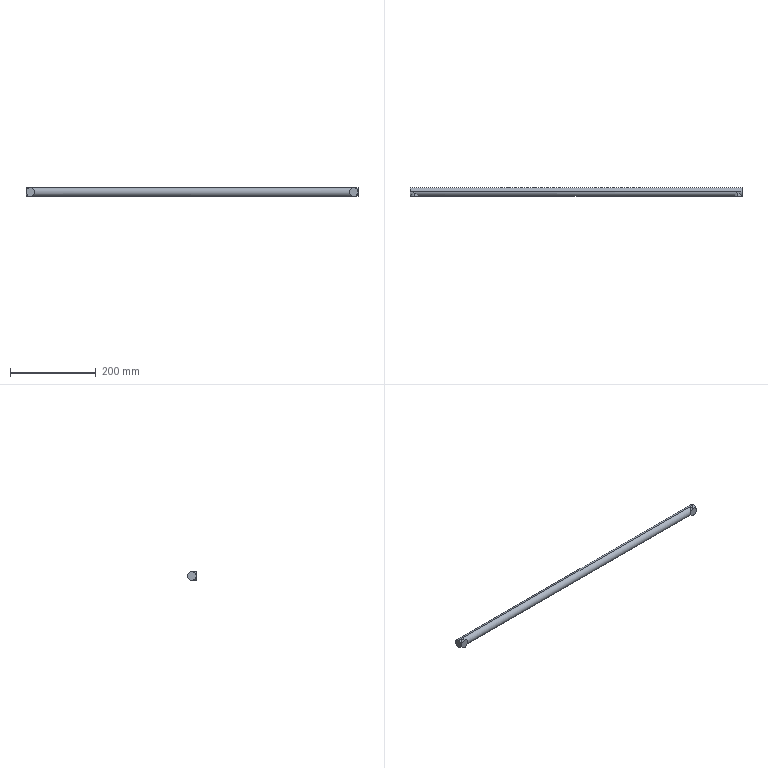Part | SolidWorks | features BaseBody 1 | 1 solid | 16 faces | box 774 x 20 x 20 mm | volume 244109 mm3 | cylinder 12 | plane 4 | commonest cylinder face diameters 20 x12
STEP:
#1=CARTESIAN_POINT('',(367.,-10.,0.));
#2=VERTEX_POINT('',#1);
#3=CARTESIAN_POINT('',(377.,-10.,10.));
#4=VERTEX_POINT('',#3);
#5=CARTESIAN_POINT('',(377.,-10.,0.));
#6=DIRECTION('',(0.,1.,0.));
#7=DIRECTION('',(0.,0.,-1.));
#8=AXIS2_PLACEMENT_3D('',#5,#6,#7);
#9=CIRCLE('',#8,10.);
#10=EDGE_CURVE('',#2,#4,#9,.T.);
#11=ORIENTED_EDGE('',*,*,#10,.F.);
#12=CARTESIAN_POINT('',(387.,-10.,0.));
#13=VERTEX_POINT('',#12);
#14=CARTESIAN_POINT('',(377.,-10.,0.));
#15=DIRECTION('',(0.,1.,0.));
#16=DIRECTION('',(0.,0.,-1.));
#17=AXIS2_PLACEMENT_3D('',#14,#15,#16);
#18=CIRCLE('',#17,10.);
#19=EDGE_CURVE('',#13,#2,#18,.T.);
#20=ORIENTED_EDGE('',*,*,#19,.F.);
#21=CARTESIAN_POINT('',(377.,-10.,0.));
#22=DIRECTION('',(0.,1.,0.));
#23=DIRECTION('',(0.,0.,-1.));
#24=AXIS2_PLACEMENT_3D('',#21,#22,#23);
#25=CIRCLE('',#24,10.);
#26=EDGE_CURVE('',#4,#13,#25,.T.);
#27=ORIENTED_EDGE('',*,*,#26,.F.);
#28=EDGE_LOOP('',(#11,#20,#27));
#29=FACE_OUTER_BOUND('',#28,.T.);
#30=CARTESIAN_POINT('',(377.,-10.,0.));
#31=DIRECTION('',(0.,-1.,0.));
#32=DIRECTION('',(0.,0.,-1.));
#33=AXIS2_PLACEMENT_3D('',#30,#31,#32);
#34=PLANE('',#33);
#35=ADVANCED_FACE('',(#29),#34,.T.);
#36=CARTESIAN_POINT('',(377.,0.,-10.));
#37=VERTEX_POINT('',#36);
#38=CARTESIAN_POINT('',(377.,0.,-10.));
#39=CARTESIAN_POINT('',(371.142,-5.858,-10.));
#40=CARTESIAN_POINT('',(367.,-10.,-5.858));
#41=CARTESIAN_POINT('',(367.,-10.,0.));
#42=(BOUNDED_CURVE()B_SPLINE_CURVE(3,(#38,#39,#40,#41),.UNSPECIFIED.,.F.,.F.)B_SPLINE_CURVE_WITH_KNOTS((4,4),(4.712,6.283),.UNSPECIFIED.)CURVE()GEOMETRIC_REPRESENTATION_ITEM()RATIONAL_B_SPLINE_CURVE((1.,0.8047,0.8047,1.))REPRESENTATION_ITEM(''));
#43=EDGE_CURVE('',#37,#2,#42,.T.);
#44=ORIENTED_EDGE('',*,*,#43,.F.);
#45=CARTESIAN_POINT('',(387.,-10.,0.));
#46=CARTESIAN_POINT('',(387.,-10.,-5.858));
#47=CARTESIAN_POINT('',(382.858,-5.858,-10.));
#48=CARTESIAN_POINT('',(377.,0.,-10.));
#49=(BOUNDED_CURVE()B_SPLINE_CURVE(3,(#45,#46,#47,#48),.UNSPECIFIED.,.F.,.F.)B_SPLINE_CURVE_WITH_KNOTS((4,4),(3.142,4.712),.UNSPECIFIED.)CURVE()GEOMETRIC_REPRESENTATION_ITEM()RATIONAL_B_SPLINE_CURVE((1.,0.8047,0.8047,1.))REPRESENTATION_ITEM(''));
#50=EDGE_CURVE('',#13,#37,#49,.T.);
#51=ORIENTED_EDGE('',*,*,#50,.F.);
#52=ORIENTED_EDGE('',*,*,#19,.T.);
#53=EDGE_LOOP('',(#44,#51,#52));
#54=FACE_OUTER_BOUND('',#53,.T.);
#55=CARTESIAN_POINT('',(377.,-10.,0.));
#56=DIRECTION('',(0.,1.,0.));
#57=DIRECTION('',(0.,0.,1.));
#58=AXIS2_PLACEMENT_3D('',#55,#56,#57);
#59=CYLINDRICAL_SURFACE('',#58,10.);
#60=ADVANCED_FACE('',(#54),#59,.T.);
#61=CARTESIAN_POINT('',(377.,0.,10.));
#62=VERTEX_POINT('',#61);
#63=CARTESIAN_POINT('',(377.,-10.,10.));
#64=DIRECTION('',(0.,1.,0.));
#65=VECTOR('',#64,1000.);
#66=LINE('',#63,#65);
#67=EDGE_CURVE('',#4,#62,#66,.T.);
#68=ORIENTED_EDGE('',*,*,#67,.F.);
#69=ORIENTED_EDGE('',*,*,#26,.T.);
#70=CARTESIAN_POINT('',(377.,0.,10.));
#71=CARTESIAN_POINT('',(382.858,-5.858,10.));
#72=CARTESIAN_POINT('',(387.,-10.,5.858));
#73=CARTESIAN_POINT('',(387.,-10.,0.));
#74=(BOUNDED_CURVE()B_SPLINE_CURVE(3,(#70,#71,#72,#73),.UNSPECIFIED.,.F.,.F.)B_SPLINE_CURVE_WITH_KNOTS((4,4),(1.571,3.142),.UNSPECIFIED.)CURVE()GEOMETRIC_REPRESENTATION_ITEM()RATIONAL_B_SPLINE_CURVE((1.,0.8047,0.8047,1.))REPRESENTATION_ITEM(''));
#75=EDGE_CURVE('',#62,#13,#74,.T.);
#76=ORIENTED_EDGE('',*,*,#75,.F.);
#77=EDGE_LOOP('',(#68,#69,#76));
#78=FACE_OUTER_BOUND('',#77,.T.);
#79=CARTESIAN_POINT('',(377.,-10.,0.));
#80=DIRECTION('',(0.,1.,0.));
#81=DIRECTION('',(0.,0.,1.));
#82=AXIS2_PLACEMENT_3D('',#79,#80,#81);
#83=CYLINDRICAL_SURFACE('',#82,10.);
#84=ADVANCED_FACE('',(#78),#83,.T.);
#85=CARTESIAN_POINT('',(-367.,-10.,0.));
#86=VERTEX_POINT('',#85);
#87=CARTESIAN_POINT('',(-387.,-10.,0.));
#88=VERTEX_POINT('',#87);
#89=CARTESIAN_POINT('',(-377.,-10.,0.));
#90=DIRECTION('',(0.,1.,0.));
#91=DIRECTION('',(0.,0.,1.));
#92=AXIS2_PLACEMENT_3D('',#89,#90,#91);
#93=CIRCLE('',#92,10.);
#94=EDGE_CURVE('',#86,#88,#93,.T.);
#95=ORIENTED_EDGE('',*,*,#94,.F.);
#96=CARTESIAN_POINT('',(-377.,-10.,10.));
#97=VERTEX_POINT('',#96);
#98=CARTESIAN_POINT('',(-377.,-10.,0.));
#99=DIRECTION('',(0.,1.,0.));
#100=DIRECTION('',(0.,0.,1.));
#101=AXIS2_PLACEMENT_3D('',#98,#99,#100);
#102=CIRCLE('',#101,10.);
#103=EDGE_CURVE('',#97,#86,#102,.T.);
#104=ORIENTED_EDGE('',*,*,#103,.F.);
#105=CARTESIAN_POINT('',(-377.,-10.,0.));
#106=DIRECTION('',(0.,1.,0.));
#107=DIRECTION('',(0.,0.,1.));
#108=AXIS2_PLACEMENT_3D('',#105,#106,#107);
#109=CIRCLE('',#108,10.);
#110=EDGE_CURVE('',#88,#97,#109,.T.);
#111=ORIENTED_EDGE('',*,*,#110,.F.);
#112=EDGE_LOOP('',(#95,#104,#111));
#113=FACE_OUTER_BOUND('',#112,.T.);
#114=CARTESIAN_POINT('',(-377.,-10.,0.));
#115=DIRECTION('',(0.,1.,0.));
#116=DIRECTION('',(1.,0.,0.));
#117=AXIS2_PLACEMENT_3D('',#114,#115,#116);
#118=PLANE('',#117);
#119=ADVANCED_FACE('',(#113),#118,.F.);
#120=CARTESIAN_POINT('',(-377.,0.,10.));
#121=VERTEX_POINT('',#120);
#122=CARTESIAN_POINT('',(-377.,-10.,10.));
#123=DIRECTION('',(0.,1.,0.));
#124=VECTOR('',#123,1000.);
#125=LINE('',#122,#124);
#126=EDGE_CURVE('',#97,#121,#125,.T.);
#127=ORIENTED_EDGE('',*,*,#126,.F.);
#128=ORIENTED_EDGE('',*,*,#103,.T.);
#129=CARTESIAN_POINT('',(-377.,0.,10.));
#130=CARTESIAN_POINT('',(-371.142,-5.858,10.));
#131=CARTESIAN_POINT('',(-367.,-10.,5.858));
#132=CARTESIAN_POINT('',(-367.,-10.,0.));
#133=(BOUNDED_CURVE()B_SPLINE_CURVE(3,(#129,#130,#131,#132),.UNSPECIFIED.,.F.,.T.)B_SPLINE_CURVE_WITH_KNOTS((4,4),(1.571,3.142),.UNSPECIFIED.)CURVE()GEOMETRIC_REPRESENTATION_ITEM()RATIONAL_B_SPLINE_CURVE((1.,0.8047,0.8047,1.))REPRESENTATION_ITEM(''));
#134=EDGE_CURVE('',#121,#86,#133,.T.);
#135=ORIENTED_EDGE('',*,*,#134,.F.);
#136=EDGE_LOOP('',(#127,#128,#135));
#137=FACE_OUTER_BOUND('',#136,.T.);
#138=CARTESIAN_POINT('',(-377.,-10.,0.));
#139=DIRECTION('',(0.,1.,0.));
#140=DIRECTION('',(0.,0.,1.));
#141=AXIS2_PLACEMENT_3D('',#138,#139,#140);
#142=CYLINDRICAL_SURFACE('',#141,10.);
#143=ADVANCED_FACE('',(#137),#142,.T.);
#144=CARTESIAN_POINT('',(-377.,0.,-10.));
#145=VERTEX_POINT('',#144);
#146=CARTESIAN_POINT('',(-377.,0.,-10.));
#147=CARTESIAN_POINT('',(-382.858,-5.858,-10.));
#148=CARTESIAN_POINT('',(-387.,-10.,-5.858));
#149=CARTESIAN_POINT('',(-387.,-10.,0.));
#150=(BOUNDED_CURVE()B_SPLINE_CURVE(3,(#146,#147,#148,#149),.UNSPECIFIED.,.F.,.F.)B_SPLINE_CURVE_WITH_KNOTS((4,4),(4.712,6.283),.UNSPECIFIED.)CURVE()GEOMETRIC_REPRESENTATION_ITEM()RATIONAL_B_SPLINE_CURVE((1.,0.8047,0.8047,1.))REPRESENTATION_ITEM(''));
#151=EDGE_CURVE('',#145,#88,#150,.T.);
#152=ORIENTED_EDGE('',*,*,#151,.F.);
#153=CARTESIAN_POINT('',(-367.,-10.,0.));
#154=CARTESIAN_POINT('',(-367.,-10.,-5.858));
#155=CARTESIAN_POINT('',(-371.142,-5.858,-10.));
#156=CARTESIAN_POINT('',(-377.,0.,-10.));
#157=(BOUNDED_CURVE()B_SPLINE_CURVE(3,(#153,#154,#155,#156),.UNSPECIFIED.,.F.,.F.)B_SPLINE_CURVE_WITH_KNOTS((4,4),(3.142,4.712),.UNSPECIFIED.)CURVE()GEOMETRIC_REPRESENTATION_ITEM()RATIONAL_B_SPLINE_CURVE((1.,0.8047,0.8047,1.))REPRESENTATION_ITEM(''));
#158=EDGE_CURVE('',#86,#145,#157,.T.);
#159=ORIENTED_EDGE('',*,*,#158,.F.);
#160=ORIENTED_EDGE('',*,*,#94,.T.);
#161=EDGE_LOOP('',(#152,#159,#160));
#162=FACE_OUTER_BOUND('',#161,.T.);
#163=CARTESIAN_POINT('',(-377.,-10.,0.));
#164=DIRECTION('',(0.,1.,0.));
#165=DIRECTION('',(0.,0.,1.));
#166=AXIS2_PLACEMENT_3D('',#163,#164,#165);
#167=CYLINDRICAL_SURFACE('',#166,10.);
#168=ADVANCED_FACE('',(#162),#167,.T.);
#169=CARTESIAN_POINT('',(-387.,0.,-10.));
#170=VERTEX_POINT('',#169);
#171=CARTESIAN_POINT('',(-387.,0.,0.));
#172=DIRECTION('',(1.,0.,0.));
#173=DIRECTION('',(0.,0.,-1.));
#174=AXIS2_PLACEMENT_3D('',#171,#172,#173);
#175=CIRCLE('',#174,10.);
#176=EDGE_CURVE('',#88,#170,#175,.T.);
#177=ORIENTED_EDGE('',*,*,#176,.F.);
#178=CARTESIAN_POINT('',(-387.,0.,10.));
#179=VERTEX_POINT('',#178);
#180=CARTESIAN_POINT('',(-387.,0.,0.));
#181=DIRECTION('',(1.,0.,0.));
#182=DIRECTION('',(0.,0.,-1.));
#183=AXIS2_PLACEMENT_3D('',#180,#181,#182);
#184=CIRCLE('',#183,10.);
#185=EDGE_CURVE('',#179,#88,#184,.T.);
#186=ORIENTED_EDGE('',*,*,#185,.F.);
#187=CARTESIAN_POINT('',(-387.,0.,0.));
#188=DIRECTION('',(1.,0.,0.));
#189=DIRECTION('',(0.,0.,-1.));
#190=AXIS2_PLACEMENT_3D('',#187,#188,#189);
#191=CIRCLE('',#190,10.);
#192=EDGE_CURVE('',#170,#179,#191,.T.);
#193=ORIENTED_EDGE('',*,*,#192,.F.);
#194=EDGE_LOOP('',(#177,#186,#193));
#195=FACE_OUTER_BOUND('',#194,.T.);
#196=CARTESIAN_POINT('',(-387.,0.,0.));
#197=DIRECTION('',(1.,0.,0.));
#198=DIRECTION('',(0.,1.,0.));
#199=AXIS2_PLACEMENT_3D('',#196,#197,#198);
#200=PLANE('',#199);
#201=ADVANCED_FACE('',(#195),#200,.F.);
#202=CARTESIAN_POINT('',(387.,0.,-10.));
#203=VERTEX_POINT('',#202);
#204=CARTESIAN_POINT('',(387.,0.,0.));
#205=DIRECTION('',(1.,0.,0.));
#206=DIRECTION('',(0.,0.,-1.));
#207=AXIS2_PLACEMENT_3D('',#204,#205,#206);
#208=CIRCLE('',#207,10.);
#209=EDGE_CURVE('',#13,#203,#208,.T.);
#210=ORIENTED_EDGE('',*,*,#209,.T.);
#211=CARTESIAN_POINT('',(387.,0.,10.));
#212=VERTEX_POINT('',#211);
#213=CARTESIAN_POINT('',(387.,0.,0.));
#214=DIRECTION('',(1.,0.,0.));
#215=DIRECTION('',(0.,0.,-1.));
#216=AXIS2_PLACEMENT_3D('',#213,#214,#215);
#217=CIRCLE('',#216,10.);
#218=EDGE_CURVE('',#203,#212,#217,.T.);
#219=ORIENTED_EDGE('',*,*,#218,.T.);
#220=CARTESIAN_POINT('',(387.,0.,0.));
#221=DIRECTION('',(1.,0.,0.));
#222=DIRECTION('',(0.,0.,-1.));
#223=AXIS2_PLACEMENT_3D('',#220,#221,#222);
#224=CIRCLE('',#223,10.);
#225=EDGE_CURVE('',#212,#13,#224,.T.);
#226=ORIENTED_EDGE('',*,*,#225,.T.);
#227=EDGE_LOOP('',(#210,#219,#226));
#228=FACE_OUTER_BOUND('',#227,.T.);
#229=CARTESIAN_POINT('',(387.,0.,0.));
#230=DIRECTION('',(1.,0.,0.));
#231=DIRECTION('',(0.,1.,0.));
#232=AXIS2_PLACEMENT_3D('',#229,#230,#231);
#233=PLANE('',#232);
#234=ADVANCED_FACE('',(#228),#233,.T.);
#235=CARTESIAN_POINT('',(387.,0.,-10.));
#236=DIRECTION('',(-1.,0.,0.));
#237=VECTOR('',#236,1000.);
#238=LINE('',#235,#237);
#239=EDGE_CURVE('',#145,#170,#238,.T.);
#240=ORIENTED_EDGE('',*,*,#239,.F.);
#241=ORIENTED_EDGE('',*,*,#151,.T.);
#242=ORIENTED_EDGE('',*,*,#176,.T.);
#243=EDGE_LOOP('',(#240,#241,#242));
#244=FACE_OUTER_BOUND('',#243,.T.);
#245=CARTESIAN_POINT('',(387.,0.,0.));
#246=DIRECTION('',(-1.,0.,0.));
#247=DIRECTION('',(0.,0.,1.));
#248=AXIS2_PLACEMENT_3D('',#245,#246,#247);
#249=CYLINDRICAL_SURFACE('',#248,10.);
#250=ADVANCED_FACE('',(#244),#249,.T.);
#251=CARTESIAN_POINT('',(-387.,-10.,0.));
#252=CARTESIAN_POINT('',(-387.,-10.,5.858));
#253=CARTESIAN_POINT('',(-382.858,-5.858,10.));
#254=CARTESIAN_POINT('',(-377.,0.,10.));
#255=(BOUNDED_CURVE()B_SPLINE_CURVE(3,(#251,#252,#253,#254),.UNSPECIFIED.,.F.,.F.)B_SPLINE_CURVE_WITH_KNOTS((4,4),(0.,1.571),.UNSPECIFIED.)CURVE()GEOMETRIC_REPRESENTATION_ITEM()RATIONAL_B_SPLINE_CURVE((1.,0.8047,0.8047,1.))REPRESENTATION_ITEM(''));
#256=EDGE_CURVE('',#88,#121,#255,.T.);
#257=ORIENTED_EDGE('',*,*,#256,.T.);
#258=CARTESIAN_POINT('',(387.,0.,10.));
#259=DIRECTION('',(-1.,0.,0.));
#260=VECTOR('',#259,1000.);
#261=LINE('',#258,#260);
#262=EDGE_CURVE('',#121,#179,#261,.T.);
#263=ORIENTED_EDGE('',*,*,#262,.T.);
#264=ORIENTED_EDGE('',*,*,#185,.T.);
#265=EDGE_LOOP('',(#257,#263,#264));
#266=FACE_OUTER_BOUND('',#265,.T.);
#267=CARTESIAN_POINT('',(387.,0.,0.));
#268=DIRECTION('',(-1.,0.,0.));
#269=DIRECTION('',(0.,0.,1.));
#270=AXIS2_PLACEMENT_3D('',#267,#268,#269);
#271=CYLINDRICAL_SURFACE('',#270,10.);
#272=ADVANCED_FACE('',(#266),#271,.T.);
#273=ORIENTED_EDGE('',*,*,#225,.F.);
#274=CARTESIAN_POINT('',(387.,0.,10.));
#275=DIRECTION('',(-1.,0.,0.));
#276=VECTOR('',#275,1000.);
#277=LINE('',#274,#276);
#278=EDGE_CURVE('',#212,#62,#277,.T.);
#279=ORIENTED_EDGE('',*,*,#278,.T.);
#280=ORIENTED_EDGE('',*,*,#75,.T.);
#281=EDGE_LOOP('',(#273,#279,#280));
#282=FACE_OUTER_BOUND('',#281,.T.);
#283=CARTESIAN_POINT('',(387.,0.,0.));
#284=DIRECTION('',(-1.,0.,0.));
#285=DIRECTION('',(0.,0.,1.));
#286=AXIS2_PLACEMENT_3D('',#283,#284,#285);
#287=CYLINDRICAL_SURFACE('',#286,10.);
#288=ADVANCED_FACE('',(#282),#287,.T.);
#289=CARTESIAN_POINT('',(387.,0.,-10.));
#290=DIRECTION('',(-1.,0.,0.));
#291=VECTOR('',#290,1000.);
#292=LINE('',#289,#291);
#293=EDGE_CURVE('',#37,#145,#292,.T.);
#294=ORIENTED_EDGE('',*,*,#293,.F.);
#295=ORIENTED_EDGE('',*,*,#43,.T.);
#296=CARTESIAN_POINT('',(367.,-10.,0.));
#297=CARTESIAN_POINT('',(367.,-10.,5.858));
#298=CARTESIAN_POINT('',(371.142,-5.858,10.));
#299=CARTESIAN_POINT('',(377.,0.,10.));
#300=(BOUNDED_CURVE()B_SPLINE_CURVE(3,(#296,#297,#298,#299),.UNSPECIFIED.,.F.,.F.)B_SPLINE_CURVE_WITH_KNOTS((4,4),(0.,1.571),.UNSPECIFIED.)CURVE()GEOMETRIC_REPRESENTATION_ITEM()RATIONAL_B_SPLINE_CURVE((1.,0.8047,0.8047,1.))REPRESENTATION_ITEM(''));
#301=EDGE_CURVE('',#2,#62,#300,.T.);
#302=ORIENTED_EDGE('',*,*,#301,.T.);
#303=CARTESIAN_POINT('',(387.,0.,10.));
#304=DIRECTION('',(-1.,0.,0.));
#305=VECTOR('',#304,1000.);
#306=LINE('',#303,#305);
#307=EDGE_CURVE('',#62,#121,#306,.T.);
#308=ORIENTED_EDGE('',*,*,#307,.T.);
#309=ORIENTED_EDGE('',*,*,#134,.T.);
#310=ORIENTED_EDGE('',*,*,#158,.T.);
#311=EDGE_LOOP('',(#294,#295,#302,#308,#309,#310));
#312=FACE_OUTER_BOUND('',#311,.T.);
#313=CARTESIAN_POINT('',(387.,0.,0.));
#314=DIRECTION('',(-1.,0.,0.));
#315=DIRECTION('',(0.,0.,1.));
#316=AXIS2_PLACEMENT_3D('',#313,#314,#315);
#317=CYLINDRICAL_SURFACE('',#316,10.);
#318=ADVANCED_FACE('',(#312),#317,.T.);
#319=CARTESIAN_POINT('',(387.,0.,-10.));
#320=DIRECTION('',(-1.,0.,0.));
#321=VECTOR('',#320,1000.);
#322=LINE('',#319,#321);
#323=EDGE_CURVE('',#203,#37,#322,.T.);
#324=ORIENTED_EDGE('',*,*,#323,.F.);
#325=ORIENTED_EDGE('',*,*,#209,.F.);
#326=ORIENTED_EDGE('',*,*,#50,.T.);
#327=EDGE_LOOP('',(#324,#325,#326));
#328=FACE_OUTER_BOUND('',#327,.T.);
#329=CARTESIAN_POINT('',(387.,0.,0.));
#330=DIRECTION('',(-1.,0.,0.));
#331=DIRECTION('',(0.,0.,1.));
#332=AXIS2_PLACEMENT_3D('',#329,#330,#331);
#333=CYLINDRICAL_SURFACE('',#332,10.);
#334=ADVANCED_FACE('',(#328),#333,.T.);
#335=ORIENTED_EDGE('',*,*,#218,.F.);
#336=ORIENTED_EDGE('',*,*,#323,.T.);
#337=ORIENTED_EDGE('',*,*,#293,.T.);
#338=ORIENTED_EDGE('',*,*,#239,.T.);
#339=ORIENTED_EDGE('',*,*,#192,.T.);
#340=ORIENTED_EDGE('',*,*,#262,.F.);
#341=ORIENTED_EDGE('',*,*,#307,.F.);
#342=ORIENTED_EDGE('',*,*,#278,.F.);
#343=EDGE_LOOP('',(#335,#336,#337,#338,#339,#340,#341,#342));
#344=FACE_OUTER_BOUND('',#343,.T.);
#345=CARTESIAN_POINT('',(387.,0.,0.));
#346=DIRECTION('',(-1.,0.,0.));
#347=DIRECTION('',(0.,0.,1.));
#348=AXIS2_PLACEMENT_3D('',#345,#346,#347);
#349=CYLINDRICAL_SURFACE('',#348,10.);
#350=ADVANCED_FACE('',(#344),#349,.T.);
#351=ORIENTED_EDGE('',*,*,#110,.T.);
#352=ORIENTED_EDGE('',*,*,#126,.T.);
#353=ORIENTED_EDGE('',*,*,#256,.F.);
#354=EDGE_LOOP('',(#351,#352,#353));
#355=FACE_OUTER_BOUND('',#354,.T.);
#356=CARTESIAN_POINT('',(-377.,-10.,0.));
#357=DIRECTION('',(0.,1.,0.));
#358=DIRECTION('',(0.,0.,1.));
#359=AXIS2_PLACEMENT_3D('',#356,#357,#358);
#360=CYLINDRICAL_SURFACE('',#359,10.);
#361=ADVANCED_FACE('',(#355),#360,.T.);
#362=ORIENTED_EDGE('',*,*,#10,.T.);
#363=ORIENTED_EDGE('',*,*,#67,.T.);
#364=ORIENTED_EDGE('',*,*,#301,.F.);
#365=EDGE_LOOP('',(#362,#363,#364));
#366=FACE_OUTER_BOUND('',#365,.T.);
#367=CARTESIAN_POINT('',(377.,-10.,0.));
#368=DIRECTION('',(0.,1.,0.));
#369=DIRECTION('',(0.,0.,1.));
#370=AXIS2_PLACEMENT_3D('',#367,#368,#369);
#371=CYLINDRICAL_SURFACE('',#370,10.);
#372=ADVANCED_FACE('',(#366),#371,.T.);
#373=CLOSED_SHELL('',(#35,#60,#84,#119,#143,#168,#201,#234,#250,#272,#288,#318,#334,#350,#361,#372));
#374=MANIFOLD_SOLID_BREP('',#373);
#375=CARTESIAN_POINT('',(0.,0.,0.));
#376=DIRECTION('',(0.,0.,1.));
#377=DIRECTION('',(1.,0.,0.));
#378=AXIS2_PLACEMENT_3D('',#375,#376,#377);
#379=(LENGTH_UNIT()NAMED_UNIT(*)SI_UNIT(.MILLI.,.METRE.));
#380=UNCERTAINTY_MEASURE_WITH_UNIT(LENGTH_MEASURE(0.00001),#379,'','');
#381=(NAMED_UNIT(*)PLANE_ANGLE_UNIT()SI_UNIT($,.RADIAN.));
#382=(NAMED_UNIT(*)SI_UNIT($,.STERADIAN.)SOLID_ANGLE_UNIT());
#383=(GEOMETRIC_REPRESENTATION_CONTEXT(3)GLOBAL_UNCERTAINTY_ASSIGNED_CONTEXT((#380))GLOBAL_UNIT_ASSIGNED_CONTEXT((#379,#381,#382))REPRESENTATION_CONTEXT('',''));
#384=ADVANCED_BREP_SHAPE_REPRESENTATION('',(#374,#378),#383);